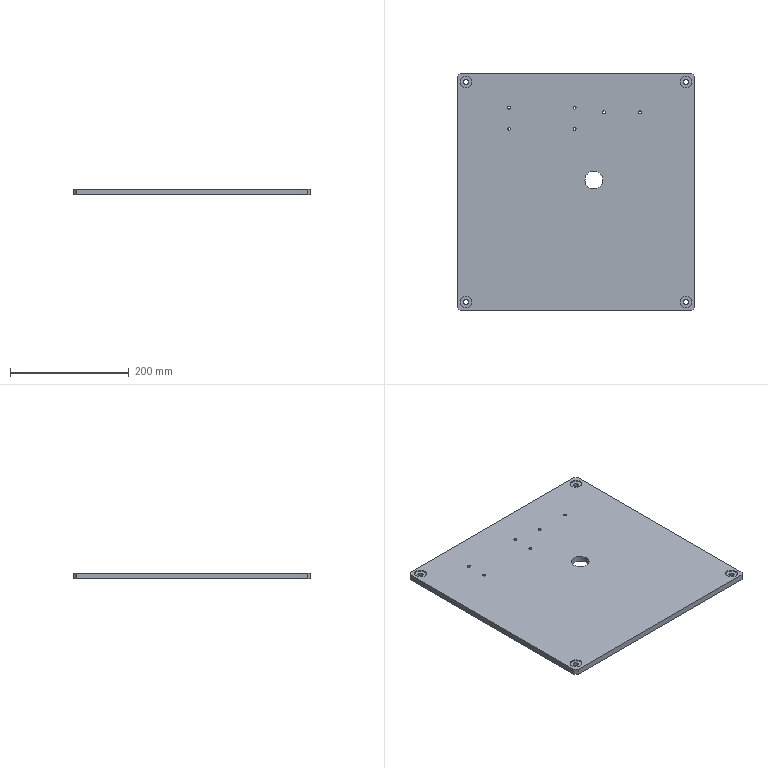Part | STEP file | 11-FG-SJ01811 | 1 solid | 44 faces | box 400 x 400 x 10 mm | volume 1586924 mm3 | cylinder 30 | plane 14 | commonest cylinder face diameters 5 x12 8.5 x8 20 x8 30 x2
STEP:
#1=CARTESIAN_POINT('',(-113.892,20.,0.));
#2=VERTEX_POINT('',#1);
#3=CARTESIAN_POINT('',(-83.892,20.,0.));
#4=VERTEX_POINT('',#3);
#5=CARTESIAN_POINT('',(-98.892,20.,0.));
#6=DIRECTION('',(0.,0.,1.));
#7=DIRECTION('',(1.,0.,0.));
#8=AXIS2_PLACEMENT_3D('',#5,#6,#7);
#9=CIRCLE('',#8,15.);
#10=EDGE_CURVE('',#2,#4,#9,.T.);
#11=ORIENTED_EDGE('',*,*,#10,.F.);
#12=CARTESIAN_POINT('',(-113.892,20.,10.));
#13=VERTEX_POINT('',#12);
#14=CARTESIAN_POINT('',(-113.892,20.,0.));
#15=DIRECTION('',(0.,0.,1.));
#16=VECTOR('',#15,1000.);
#17=LINE('',#14,#16);
#18=EDGE_CURVE('',#2,#13,#17,.T.);
#19=ORIENTED_EDGE('',*,*,#18,.T.);
#20=CARTESIAN_POINT('',(-83.892,20.,10.));
#21=VERTEX_POINT('',#20);
#22=CARTESIAN_POINT('',(-98.892,20.,10.));
#23=DIRECTION('',(0.,0.,1.));
#24=DIRECTION('',(1.,0.,0.));
#25=AXIS2_PLACEMENT_3D('',#22,#23,#24);
#26=CIRCLE('',#25,15.);
#27=EDGE_CURVE('',#13,#21,#26,.T.);
#28=ORIENTED_EDGE('',*,*,#27,.T.);
#29=CARTESIAN_POINT('',(-83.892,20.,0.));
#30=DIRECTION('',(0.,0.,1.));
#31=VECTOR('',#30,1000.);
#32=LINE('',#29,#31);
#33=EDGE_CURVE('',#4,#21,#32,.T.);
#34=ORIENTED_EDGE('',*,*,#33,.F.);
#35=EDGE_LOOP('',(#11,#19,#28,#34));
#36=FACE_OUTER_BOUND('',#35,.T.);
#37=CARTESIAN_POINT('',(-98.892,20.,0.));
#38=DIRECTION('',(0.,0.,1.));
#39=DIRECTION('',(1.,0.,0.));
#40=AXIS2_PLACEMENT_3D('',#37,#38,#39);
#41=CYLINDRICAL_SURFACE('',#40,15.);
#42=ADVANCED_FACE('',(#36),#41,.F.);
#43=CARTESIAN_POINT('',(-23.892,134.,0.));
#44=VERTEX_POINT('',#43);
#45=CARTESIAN_POINT('',(-18.892,134.,0.));
#46=VERTEX_POINT('',#45);
#47=CARTESIAN_POINT('',(-21.392,134.,0.));
#48=DIRECTION('',(0.,0.,1.));
#49=DIRECTION('',(1.,0.,0.));
#50=AXIS2_PLACEMENT_3D('',#47,#48,#49);
#51=CIRCLE('',#50,2.5);
#52=EDGE_CURVE('',#44,#46,#51,.T.);
#53=ORIENTED_EDGE('',*,*,#52,.F.);
#54=CARTESIAN_POINT('',(-23.892,134.,10.));
#55=VERTEX_POINT('',#54);
#56=CARTESIAN_POINT('',(-23.892,134.,10.));
#57=DIRECTION('',(0.,0.,1.));
#58=VECTOR('',#57,1000.);
#59=LINE('',#56,#58);
#60=EDGE_CURVE('',#44,#55,#59,.T.);
#61=ORIENTED_EDGE('',*,*,#60,.T.);
#62=CARTESIAN_POINT('',(-18.892,134.,10.));
#63=VERTEX_POINT('',#62);
#64=CARTESIAN_POINT('',(-21.392,134.,10.));
#65=DIRECTION('',(0.,0.,1.));
#66=DIRECTION('',(1.,0.,0.));
#67=AXIS2_PLACEMENT_3D('',#64,#65,#66);
#68=CIRCLE('',#67,2.5);
#69=EDGE_CURVE('',#55,#63,#68,.T.);
#70=ORIENTED_EDGE('',*,*,#69,.T.);
#71=CARTESIAN_POINT('',(-18.892,134.,10.));
#72=DIRECTION('',(0.,0.,1.));
#73=VECTOR('',#72,1000.);
#74=LINE('',#71,#73);
#75=EDGE_CURVE('',#46,#63,#74,.T.);
#76=ORIENTED_EDGE('',*,*,#75,.F.);
#77=EDGE_LOOP('',(#53,#61,#70,#76));
#78=FACE_OUTER_BOUND('',#77,.T.);
#79=CARTESIAN_POINT('',(-21.392,134.,10.));
#80=DIRECTION('',(0.,0.,1.));
#81=DIRECTION('',(1.,0.,0.));
#82=AXIS2_PLACEMENT_3D('',#79,#80,#81);
#83=CYLINDRICAL_SURFACE('',#82,2.5);
#84=ADVANCED_FACE('',(#78),#83,.F.);
#85=CARTESIAN_POINT('',(-83.892,134.,0.));
#86=VERTEX_POINT('',#85);
#87=CARTESIAN_POINT('',(-78.892,134.,0.));
#88=VERTEX_POINT('',#87);
#89=CARTESIAN_POINT('',(-81.392,134.,0.));
#90=DIRECTION('',(0.,0.,1.));
#91=DIRECTION('',(1.,0.,0.));
#92=AXIS2_PLACEMENT_3D('',#89,#90,#91);
#93=CIRCLE('',#92,2.5);
#94=EDGE_CURVE('',#86,#88,#93,.T.);
#95=ORIENTED_EDGE('',*,*,#94,.F.);
#96=CARTESIAN_POINT('',(-83.892,134.,10.));
#97=VERTEX_POINT('',#96);
#98=CARTESIAN_POINT('',(-83.892,134.,10.));
#99=DIRECTION('',(0.,0.,1.));
#100=VECTOR('',#99,1000.);
#101=LINE('',#98,#100);
#102=EDGE_CURVE('',#86,#97,#101,.T.);
#103=ORIENTED_EDGE('',*,*,#102,.T.);
#104=CARTESIAN_POINT('',(-78.892,134.,10.));
#105=VERTEX_POINT('',#104);
#106=CARTESIAN_POINT('',(-81.392,134.,10.));
#107=DIRECTION('',(0.,0.,1.));
#108=DIRECTION('',(1.,0.,0.));
#109=AXIS2_PLACEMENT_3D('',#106,#107,#108);
#110=CIRCLE('',#109,2.5);
#111=EDGE_CURVE('',#97,#105,#110,.T.);
#112=ORIENTED_EDGE('',*,*,#111,.T.);
#113=CARTESIAN_POINT('',(-78.892,134.,10.));
#114=DIRECTION('',(0.,0.,1.));
#115=VECTOR('',#114,1000.);
#116=LINE('',#113,#115);
#117=EDGE_CURVE('',#88,#105,#116,.T.);
#118=ORIENTED_EDGE('',*,*,#117,.F.);
#119=EDGE_LOOP('',(#95,#103,#112,#118));
#120=FACE_OUTER_BOUND('',#119,.T.);
#121=CARTESIAN_POINT('',(-81.392,134.,10.));
#122=DIRECTION('',(0.,0.,1.));
#123=DIRECTION('',(1.,0.,0.));
#124=AXIS2_PLACEMENT_3D('',#121,#122,#123);
#125=CYLINDRICAL_SURFACE('',#124,2.5);
#126=ADVANCED_FACE('',(#120),#125,.F.);
#127=CARTESIAN_POINT('',(-133.892,142.,0.));
#128=VERTEX_POINT('',#127);
#129=CARTESIAN_POINT('',(-128.892,142.,0.));
#130=VERTEX_POINT('',#129);
#131=CARTESIAN_POINT('',(-131.392,142.,0.));
#132=DIRECTION('',(0.,0.,1.));
#133=DIRECTION('',(1.,0.,0.));
#134=AXIS2_PLACEMENT_3D('',#131,#132,#133);
#135=CIRCLE('',#134,2.5);
#136=EDGE_CURVE('',#128,#130,#135,.T.);
#137=ORIENTED_EDGE('',*,*,#136,.F.);
#138=CARTESIAN_POINT('',(-133.892,142.,10.));
#139=VERTEX_POINT('',#138);
#140=CARTESIAN_POINT('',(-133.892,142.,10.));
#141=DIRECTION('',(0.,0.,1.));
#142=VECTOR('',#141,1000.);
#143=LINE('',#140,#142);
#144=EDGE_CURVE('',#128,#139,#143,.T.);
#145=ORIENTED_EDGE('',*,*,#144,.T.);
#146=CARTESIAN_POINT('',(-128.892,142.,10.));
#147=VERTEX_POINT('',#146);
#148=CARTESIAN_POINT('',(-131.392,142.,10.));
#149=DIRECTION('',(0.,0.,1.));
#150=DIRECTION('',(1.,0.,0.));
#151=AXIS2_PLACEMENT_3D('',#148,#149,#150);
#152=CIRCLE('',#151,2.5);
#153=EDGE_CURVE('',#139,#147,#152,.T.);
#154=ORIENTED_EDGE('',*,*,#153,.T.);
#155=CARTESIAN_POINT('',(-128.892,142.,10.));
#156=DIRECTION('',(0.,0.,1.));
#157=VECTOR('',#156,1000.);
#158=LINE('',#155,#157);
#159=EDGE_CURVE('',#130,#147,#158,.T.);
#160=ORIENTED_EDGE('',*,*,#159,.F.);
#161=EDGE_LOOP('',(#137,#145,#154,#160));
#162=FACE_OUTER_BOUND('',#161,.T.);
#163=CARTESIAN_POINT('',(-131.392,142.,10.));
#164=DIRECTION('',(0.,0.,1.));
#165=DIRECTION('',(1.,0.,0.));
#166=AXIS2_PLACEMENT_3D('',#163,#164,#165);
#167=CYLINDRICAL_SURFACE('',#166,2.5);
#168=ADVANCED_FACE('',(#162),#167,.F.);
#169=CARTESIAN_POINT('',(-133.892,106.,0.));
#170=VERTEX_POINT('',#169);
#171=CARTESIAN_POINT('',(-128.892,106.,0.));
#172=VERTEX_POINT('',#171);
#173=CARTESIAN_POINT('',(-131.392,106.,0.));
#174=DIRECTION('',(0.,0.,1.));
#175=DIRECTION('',(1.,0.,0.));
#176=AXIS2_PLACEMENT_3D('',#173,#174,#175);
#177=CIRCLE('',#176,2.5);
#178=EDGE_CURVE('',#170,#172,#177,.T.);
#179=ORIENTED_EDGE('',*,*,#178,.F.);
#180=CARTESIAN_POINT('',(-133.892,106.,10.));
#181=VERTEX_POINT('',#180);
#182=CARTESIAN_POINT('',(-133.892,106.,10.));
#183=DIRECTION('',(0.,0.,1.));
#184=VECTOR('',#183,1000.);
#185=LINE('',#182,#184);
#186=EDGE_CURVE('',#170,#181,#185,.T.);
#187=ORIENTED_EDGE('',*,*,#186,.T.);
#188=CARTESIAN_POINT('',(-128.892,106.,10.));
#189=VERTEX_POINT('',#188);
#190=CARTESIAN_POINT('',(-131.392,106.,10.));
#191=DIRECTION('',(0.,0.,1.));
#192=DIRECTION('',(1.,0.,0.));
#193=AXIS2_PLACEMENT_3D('',#190,#191,#192);
#194=CIRCLE('',#193,2.5);
#195=EDGE_CURVE('',#181,#189,#194,.T.);
#196=ORIENTED_EDGE('',*,*,#195,.T.);
#197=CARTESIAN_POINT('',(-128.892,106.,10.));
#198=DIRECTION('',(0.,0.,1.));
#199=VECTOR('',#198,1000.);
#200=LINE('',#197,#199);
#201=EDGE_CURVE('',#172,#189,#200,.T.);
#202=ORIENTED_EDGE('',*,*,#201,.F.);
#203=EDGE_LOOP('',(#179,#187,#196,#202));
#204=FACE_OUTER_BOUND('',#203,.T.);
#205=CARTESIAN_POINT('',(-131.392,106.,10.));
#206=DIRECTION('',(0.,0.,1.));
#207=DIRECTION('',(1.,0.,0.));
#208=AXIS2_PLACEMENT_3D('',#205,#206,#207);
#209=CYLINDRICAL_SURFACE('',#208,2.5);
#210=ADVANCED_FACE('',(#204),#209,.F.);
#211=CARTESIAN_POINT('',(-243.892,106.,0.));
#212=VERTEX_POINT('',#211);
#213=CARTESIAN_POINT('',(-238.892,106.,0.));
#214=VERTEX_POINT('',#213);
#215=CARTESIAN_POINT('',(-241.392,106.,0.));
#216=DIRECTION('',(0.,0.,1.));
#217=DIRECTION('',(1.,0.,0.));
#218=AXIS2_PLACEMENT_3D('',#215,#216,#217);
#219=CIRCLE('',#218,2.5);
#220=EDGE_CURVE('',#212,#214,#219,.T.);
#221=ORIENTED_EDGE('',*,*,#220,.F.);
#222=CARTESIAN_POINT('',(-243.892,106.,10.));
#223=VERTEX_POINT('',#222);
#224=CARTESIAN_POINT('',(-243.892,106.,10.));
#225=DIRECTION('',(0.,0.,1.));
#226=VECTOR('',#225,1000.);
#227=LINE('',#224,#226);
#228=EDGE_CURVE('',#212,#223,#227,.T.);
#229=ORIENTED_EDGE('',*,*,#228,.T.);
#230=CARTESIAN_POINT('',(-238.892,106.,10.));
#231=VERTEX_POINT('',#230);
#232=CARTESIAN_POINT('',(-241.392,106.,10.));
#233=DIRECTION('',(0.,0.,1.));
#234=DIRECTION('',(1.,0.,0.));
#235=AXIS2_PLACEMENT_3D('',#232,#233,#234);
#236=CIRCLE('',#235,2.5);
#237=EDGE_CURVE('',#223,#231,#236,.T.);
#238=ORIENTED_EDGE('',*,*,#237,.T.);
#239=CARTESIAN_POINT('',(-238.892,106.,10.));
#240=DIRECTION('',(0.,0.,1.));
#241=VECTOR('',#240,1000.);
#242=LINE('',#239,#241);
#243=EDGE_CURVE('',#214,#231,#242,.T.);
#244=ORIENTED_EDGE('',*,*,#243,.F.);
#245=EDGE_LOOP('',(#221,#229,#238,#244));
#246=FACE_OUTER_BOUND('',#245,.T.);
#247=CARTESIAN_POINT('',(-241.392,106.,10.));
#248=DIRECTION('',(0.,0.,1.));
#249=DIRECTION('',(1.,0.,0.));
#250=AXIS2_PLACEMENT_3D('',#247,#248,#249);
#251=CYLINDRICAL_SURFACE('',#250,2.5);
#252=ADVANCED_FACE('',(#246),#251,.F.);
#253=CARTESIAN_POINT('',(-243.892,142.,0.));
#254=VERTEX_POINT('',#253);
#255=CARTESIAN_POINT('',(-238.892,142.,0.));
#256=VERTEX_POINT('',#255);
#257=CARTESIAN_POINT('',(-241.392,142.,0.));
#258=DIRECTION('',(0.,0.,1.));
#259=DIRECTION('',(1.,0.,0.));
#260=AXIS2_PLACEMENT_3D('',#257,#258,#259);
#261=CIRCLE('',#260,2.5);
#262=EDGE_CURVE('',#254,#256,#261,.T.);
#263=ORIENTED_EDGE('',*,*,#262,.F.);
#264=CARTESIAN_POINT('',(-243.892,142.,10.));
#265=VERTEX_POINT('',#264);
#266=CARTESIAN_POINT('',(-243.892,142.,10.));
#267=DIRECTION('',(0.,0.,1.));
#268=VECTOR('',#267,1000.);
#269=LINE('',#266,#268);
#270=EDGE_CURVE('',#254,#265,#269,.T.);
#271=ORIENTED_EDGE('',*,*,#270,.T.);
#272=CARTESIAN_POINT('',(-238.892,142.,10.));
#273=VERTEX_POINT('',#272);
#274=CARTESIAN_POINT('',(-241.392,142.,10.));
#275=DIRECTION('',(0.,0.,1.));
#276=DIRECTION('',(1.,0.,0.));
#277=AXIS2_PLACEMENT_3D('',#274,#275,#276);
#278=CIRCLE('',#277,2.5);
#279=EDGE_CURVE('',#265,#273,#278,.T.);
#280=ORIENTED_EDGE('',*,*,#279,.T.);
#281=CARTESIAN_POINT('',(-238.892,142.,10.));
#282=DIRECTION('',(0.,0.,1.));
#283=VECTOR('',#282,1000.);
#284=LINE('',#281,#283);
#285=EDGE_CURVE('',#256,#273,#284,.T.);
#286=ORIENTED_EDGE('',*,*,#285,.F.);
#287=EDGE_LOOP('',(#263,#271,#280,#286));
#288=FACE_OUTER_BOUND('',#287,.T.);
#289=CARTESIAN_POINT('',(-241.392,142.,10.));
#290=DIRECTION('',(0.,0.,1.));
#291=DIRECTION('',(1.,0.,0.));
#292=AXIS2_PLACEMENT_3D('',#289,#290,#291);
#293=CYLINDRICAL_SURFACE('',#292,2.5);
#294=ADVANCED_FACE('',(#288),#293,.F.);
#295=CARTESIAN_POINT('',(-318.142,-185.,0.));
#296=VERTEX_POINT('',#295);
#297=CARTESIAN_POINT('',(-309.642,-185.,0.));
#298=VERTEX_POINT('',#297);
#299=CARTESIAN_POINT('',(-313.892,-185.,0.));
#300=DIRECTION('',(0.,0.,1.));
#301=DIRECTION('',(1.,0.,0.));
#302=AXIS2_PLACEMENT_3D('',#299,#300,#301);
#303=CIRCLE('',#302,4.25);
#304=EDGE_CURVE('',#296,#298,#303,.T.);
#305=ORIENTED_EDGE('',*,*,#304,.F.);
#306=CARTESIAN_POINT('',(-318.142,-185.,8.));
#307=VERTEX_POINT('',#306);
#308=CARTESIAN_POINT('',(-318.142,-185.,0.));
#309=DIRECTION('',(0.,0.,1.));
#310=VECTOR('',#309,1000.);
#311=LINE('',#308,#310);
#312=EDGE_CURVE('',#296,#307,#311,.T.);
#313=ORIENTED_EDGE('',*,*,#312,.T.);
#314=CARTESIAN_POINT('',(-309.642,-185.,8.));
#315=VERTEX_POINT('',#314);
#316=CARTESIAN_POINT('',(-313.892,-185.,8.));
#317=DIRECTION('',(0.,0.,-1.));
#318=DIRECTION('',(-1.,0.,0.));
#319=AXIS2_PLACEMENT_3D('',#316,#317,#318);
#320=CIRCLE('',#319,4.25);
#321=EDGE_CURVE('',#315,#307,#320,.T.);
#322=ORIENTED_EDGE('',*,*,#321,.F.);
#323=CARTESIAN_POINT('',(-309.642,-185.,0.));
#324=DIRECTION('',(0.,0.,1.));
#325=VECTOR('',#324,1000.);
#326=LINE('',#323,#325);
#327=EDGE_CURVE('',#298,#315,#326,.T.);
#328=ORIENTED_EDGE('',*,*,#327,.F.);
#329=EDGE_LOOP('',(#305,#313,#322,#328));
#330=FACE_OUTER_BOUND('',#329,.T.);
#331=CARTESIAN_POINT('',(-313.892,-185.,0.));
#332=DIRECTION('',(0.,0.,1.));
#333=DIRECTION('',(1.,0.,0.));
#334=AXIS2_PLACEMENT_3D('',#331,#332,#333);
#335=CYLINDRICAL_SURFACE('',#334,4.25);
#336=ADVANCED_FACE('',(#330),#335,.F.);
#337=CARTESIAN_POINT('',(51.858,-185.,0.));
#338=VERTEX_POINT('',#337);
#339=CARTESIAN_POINT('',(60.358,-185.,0.));
#340=VERTEX_POINT('',#339);
#341=CARTESIAN_POINT('',(56.108,-185.,0.));
#342=DIRECTION('',(0.,0.,1.));
#343=DIRECTION('',(1.,0.,0.));
#344=AXIS2_PLACEMENT_3D('',#341,#342,#343);
#345=CIRCLE('',#344,4.25);
#346=EDGE_CURVE('',#338,#340,#345,.T.);
#347=ORIENTED_EDGE('',*,*,#346,.F.);
#348=CARTESIAN_POINT('',(51.858,-185.,8.));
#349=VERTEX_POINT('',#348);
#350=CARTESIAN_POINT('',(51.858,-185.,0.));
#351=DIRECTION('',(0.,0.,1.));
#352=VECTOR('',#351,1000.);
#353=LINE('',#350,#352);
#354=EDGE_CURVE('',#338,#349,#353,.T.);
#355=ORIENTED_EDGE('',*,*,#354,.T.);
#356=CARTESIAN_POINT('',(60.358,-185.,8.));
#357=VERTEX_POINT('',#356);
#358=CARTESIAN_POINT('',(56.108,-185.,8.));
#359=DIRECTION('',(0.,0.,1.));
#360=DIRECTION('',(1.,0.,0.));
#361=AXIS2_PLACEMENT_3D('',#358,#359,#360);
#362=CIRCLE('',#361,4.25);
#363=EDGE_CURVE('',#349,#357,#362,.T.);
#364=ORIENTED_EDGE('',*,*,#363,.T.);
#365=CARTESIAN_POINT('',(60.358,-185.,0.));
#366=DIRECTION('',(0.,0.,1.));
#367=VECTOR('',#366,1000.);
#368=LINE('',#365,#367);
#369=EDGE_CURVE('',#340,#357,#368,.T.);
#370=ORIENTED_EDGE('',*,*,#369,.F.);
#371=EDGE_LOOP('',(#347,#355,#364,#370));
#372=FACE_OUTER_BOUND('',#371,.T.);
#373=CARTESIAN_POINT('',(56.108,-185.,0.));
#374=DIRECTION('',(0.,0.,1.));
#375=DIRECTION('',(1.,0.,0.));
#376=AXIS2_PLACEMENT_3D('',#373,#374,#375);
#377=CYLINDRICAL_SURFACE('',#376,4.25);
#378=ADVANCED_FACE('',(#372),#377,.F.);
#379=CARTESIAN_POINT('',(51.858,185.,0.));
#380=VERTEX_POINT('',#379);
#381=CARTESIAN_POINT('',(60.358,185.,0.));
#382=VERTEX_POINT('',#381);
#383=CARTESIAN_POINT('',(56.108,185.,0.));
#384=DIRECTION('',(0.,0.,1.));
#385=DIRECTION('',(1.,0.,0.));
#386=AXIS2_PLACEMENT_3D('',#383,#384,#385);
#387=CIRCLE('',#386,4.25);
#388=EDGE_CURVE('',#380,#382,#387,.T.);
#389=ORIENTED_EDGE('',*,*,#388,.F.);
#390=CARTESIAN_POINT('',(51.858,185.,8.));
#391=VERTEX_POINT('',#390);
#392=CARTESIAN_POINT('',(51.858,185.,0.));
#393=DIRECTION('',(0.,0.,1.));
#394=VECTOR('',#393,1000.);
#395=LINE('',#392,#394);
#396=EDGE_CURVE('',#380,#391,#395,.T.);
#397=ORIENTED_EDGE('',*,*,#396,.T.);
#398=CARTESIAN_POINT('',(60.358,185.,8.));
#399=VERTEX_POINT('',#398);
#400=CARTESIAN_POINT('',(56.108,185.,8.));
#401=DIRECTION('',(0.,0.,-1.));
#402=DIRECTION('',(-1.,0.,0.));
#403=AXIS2_PLACEMENT_3D('',#400,#401,#402);
#404=CIRCLE('',#403,4.25);
#405=EDGE_CURVE('',#399,#391,#404,.T.);
#406=ORIENTED_EDGE('',*,*,#405,.F.);
#407=CARTESIAN_POINT('',(60.358,185.,0.));
#408=DIRECTION('',(0.,0.,1.));
#409=VECTOR('',#408,1000.);
#410=LINE('',#407,#409);
#411=EDGE_CURVE('',#382,#399,#410,.T.);
#412=ORIENTED_EDGE('',*,*,#411,.F.);
#413=EDGE_LOOP('',(#389,#397,#406,#412));
#414=FACE_OUTER_BOUND('',#413,.T.);
#415=CARTESIAN_POINT('',(56.108,185.,0.));
#416=DIRECTION('',(0.,0.,1.));
#417=DIRECTION('',(1.,0.,0.));
#418=AXIS2_PLACEMENT_3D('',#415,#416,#417);
#419=CYLINDRICAL_SURFACE('',#418,4.25);
#420=ADVANCED_FACE('',(#414),#419,.F.);
#421=CARTESIAN_POINT('',(-318.142,185.,0.));
#422=VERTEX_POINT('',#421);
#423=CARTESIAN_POINT('',(-309.642,185.,0.));
#424=VERTEX_POINT('',#423);
#425=CARTESIAN_POINT('',(-313.892,185.,0.));
#426=DIRECTION('',(0.,0.,1.));
#427=DIRECTION('',(1.,0.,0.));
#428=AXIS2_PLACEMENT_3D('',#425,#426,#427);
#429=CIRCLE('',#428,4.25);
#430=EDGE_CURVE('',#422,#424,#429,.T.);
#431=ORIENTED_EDGE('',*,*,#430,.F.);
#432=CARTESIAN_POINT('',(-318.142,185.,8.));
#433=VERTEX_POINT('',#432);
#434=CARTESIAN_POINT('',(-318.142,185.,0.));
#435=DIRECTION('',(0.,0.,1.));
#436=VECTOR('',#435,1000.);
#437=LINE('',#434,#436);
#438=EDGE_CURVE('',#422,#433,#437,.T.);
#439=ORIENTED_EDGE('',*,*,#438,.T.);
#440=CARTESIAN_POINT('',(-309.642,185.,8.));
#441=VERTEX_POINT('',#440);
#442=CARTESIAN_POINT('',(-313.892,185.,8.));
#443=DIRECTION('',(0.,0.,1.));
#444=DIRECTION('',(1.,0.,0.));
#445=AXIS2_PLACEMENT_3D('',#442,#443,#444);
#446=CIRCLE('',#445,4.25);
#447=EDGE_CURVE('',#433,#441,#446,.T.);
#448=ORIENTED_EDGE('',*,*,#447,.T.);
#449=CARTESIAN_POINT('',(-309.642,185.,0.));
#450=DIRECTION('',(0.,0.,1.));
#451=VECTOR('',#450,1000.);
#452=LINE('',#449,#451);
#453=EDGE_CURVE('',#424,#441,#452,.T.);
#454=ORIENTED_EDGE('',*,*,#453,.F.);
#455=EDGE_LOOP('',(#431,#439,#448,#454));
#456=FACE_OUTER_BOUND('',#455,.T.);
#457=CARTESIAN_POINT('',(-313.892,185.,0.));
#458=DIRECTION('',(0.,0.,1.));
#459=DIRECTION('',(1.,0.,0.));
#460=AXIS2_PLACEMENT_3D('',#457,#458,#459);
#461=CYLINDRICAL_SURFACE('',#460,4.25);
#462=ADVANCED_FACE('',(#456),#461,.F.);
#463=CARTESIAN_POINT('',(46.108,185.,8.));
#464=VERTEX_POINT('',#463);
#465=CARTESIAN_POINT('',(66.108,185.,8.));
#466=VERTEX_POINT('',#465);
#467=CARTESIAN_POINT('',(56.108,185.,8.));
#468=DIRECTION('',(0.,0.,1.));
#469=DIRECTION('',(-1.,0.,0.));
#470=AXIS2_PLACEMENT_3D('',#467,#468,#469);
#471=CIRCLE('',#470,10.);
#472=EDGE_CURVE('',#464,#466,#471,.T.);
#473=ORIENTED_EDGE('',*,*,#472,.F.);
#474=CARTESIAN_POINT('',(46.108,185.,10.));
#475=VERTEX_POINT('',#474);
#476=CARTESIAN_POINT('',(46.108,185.,8.));
#477=DIRECTION('',(0.,0.,1.));
#478=VECTOR('',#477,1000.);
#479=LINE('',#476,#478);
#480=EDGE_CURVE('',#464,#475,#479,.T.);
#481=ORIENTED_EDGE('',*,*,#480,.T.);
#482=CARTESIAN_POINT('',(66.108,185.,10.));
#483=VERTEX_POINT('',#482);
#484=CARTESIAN_POINT('',(56.108,185.,10.));
#485=DIRECTION('',(0.,0.,1.));
#486=DIRECTION('',(-1.,0.,0.));
#487=AXIS2_PLACEMENT_3D('',#484,#485,#486);
#488=CIRCLE('',#487,10.);
#489=EDGE_CURVE('',#475,#483,#488,.T.);
#490=ORIENTED_EDGE('',*,*,#489,.T.);
#491=CARTESIAN_POINT('',(66.108,185.,8.));
#492=DIRECTION('',(0.,0.,1.));
#493=VECTOR('',#492,1000.);
#494=LINE('',#491,#493);
#495=EDGE_CURVE('',#466,#483,#494,.T.);
#496=ORIENTED_EDGE('',*,*,#495,.F.);
#497=EDGE_LOOP('',(#473,#481,#490,#496));
#498=FACE_OUTER_BOUND('',#497,.T.);
#499=CARTESIAN_POINT('',(56.108,185.,8.));
#500=DIRECTION('',(0.,0.,1.));
#501=DIRECTION('',(1.,0.,0.));
#502=AXIS2_PLACEMENT_3D('',#499,#500,#501);
#503=CYLINDRICAL_SURFACE('',#502,10.);
#504=ADVANCED_FACE('',(#498),#503,.F.);
#505=CARTESIAN_POINT('',(46.108,-185.,8.));
#506=VERTEX_POINT('',#505);
#507=CARTESIAN_POINT('',(66.108,-185.,8.));
#508=VERTEX_POINT('',#507);
#509=CARTESIAN_POINT('',(56.108,-185.,8.));
#510=DIRECTION('',(0.,0.,1.));
#511=DIRECTION('',(1.,0.,0.));
#512=AXIS2_PLACEMENT_3D('',#509,#510,#511);
#513=CIRCLE('',#512,10.);
#514=EDGE_CURVE('',#506,#508,#513,.T.);
#515=ORIENTED_EDGE('',*,*,#514,.F.);
#516=CARTESIAN_POINT('',(46.108,-185.,10.));
#517=VERTEX_POINT('',#516);
#518=CARTESIAN_POINT('',(46.108,-185.,8.));
#519=DIRECTION('',(0.,0.,1.));
#520=VECTOR('',#519,1000.);
#521=LINE('',#518,#520);
#522=EDGE_CURVE('',#506,#517,#521,.T.);
#523=ORIENTED_EDGE('',*,*,#522,.T.);
#524=CARTESIAN_POINT('',(66.108,-185.,10.));
#525=VERTEX_POINT('',#524);
#526=CARTESIAN_POINT('',(56.108,-185.,10.));
#527=DIRECTION('',(0.,0.,1.));
#528=DIRECTION('',(1.,0.,0.));
#529=AXIS2_PLACEMENT_3D('',#526,#527,#528);
#530=CIRCLE('',#529,10.);
#531=EDGE_CURVE('',#517,#525,#530,.T.);
#532=ORIENTED_EDGE('',*,*,#531,.T.);
#533=CARTESIAN_POINT('',(66.108,-185.,8.));
#534=DIRECTION('',(0.,0.,1.));
#535=VECTOR('',#534,1000.);
#536=LINE('',#533,#535);
#537=EDGE_CURVE('',#508,#525,#536,.T.);
#538=ORIENTED_EDGE('',*,*,#537,.F.);
#539=EDGE_LOOP('',(#515,#523,#532,#538));
#540=FACE_OUTER_BOUND('',#539,.T.);
#541=CARTESIAN_POINT('',(56.108,-185.,8.));
#542=DIRECTION('',(0.,0.,1.));
#543=DIRECTION('',(1.,0.,0.));
#544=AXIS2_PLACEMENT_3D('',#541,#542,#543);
#545=CYLINDRICAL_SURFACE('',#544,10.);
#546=ADVANCED_FACE('',(#540),#545,.F.);
#547=CARTESIAN_POINT('',(-323.892,-185.,8.));
#548=VERTEX_POINT('',#547);
#549=CARTESIAN_POINT('',(-303.892,-185.,8.));
#550=VERTEX_POINT('',#549);
#551=CARTESIAN_POINT('',(-313.892,-185.,8.));
#552=DIRECTION('',(0.,0.,1.));
#553=DIRECTION('',(-1.,0.,0.));
#554=AXIS2_PLACEMENT_3D('',#551,#552,#553);
#555=CIRCLE('',#554,10.);
#556=EDGE_CURVE('',#548,#550,#555,.T.);
#557=ORIENTED_EDGE('',*,*,#556,.F.);
#558=CARTESIAN_POINT('',(-323.892,-185.,10.));
#559=VERTEX_POINT('',#558);
#560=CARTESIAN_POINT('',(-323.892,-185.,8.));
#561=DIRECTION('',(0.,0.,1.));
#562=VECTOR('',#561,1000.);
#563=LINE('',#560,#562);
#564=EDGE_CURVE('',#548,#559,#563,.T.);
#565=ORIENTED_EDGE('',*,*,#564,.T.);
#566=CARTESIAN_POINT('',(-303.892,-185.,10.));
#567=VERTEX_POINT('',#566);
#568=CARTESIAN_POINT('',(-313.892,-185.,10.));
#569=DIRECTION('',(0.,0.,1.));
#570=DIRECTION('',(-1.,0.,0.));
#571=AXIS2_PLACEMENT_3D('',#568,#569,#570);
#572=CIRCLE('',#571,10.);
#573=EDGE_CURVE('',#559,#567,#572,.T.);
#574=ORIENTED_EDGE('',*,*,#573,.T.);
#575=CARTESIAN_POINT('',(-303.892,-185.,8.));
#576=DIRECTION('',(0.,0.,1.));
#577=VECTOR('',#576,1000.);
#578=LINE('',#575,#577);
#579=EDGE_CURVE('',#550,#567,#578,.T.);
#580=ORIENTED_EDGE('',*,*,#579,.F.);
#581=EDGE_LOOP('',(#557,#565,#574,#580));
#582=FACE_OUTER_BOUND('',#581,.T.);
#583=CARTESIAN_POINT('',(-313.892,-185.,8.));
#584=DIRECTION('',(0.,0.,1.));
#585=DIRECTION('',(1.,0.,0.));
#586=AXIS2_PLACEMENT_3D('',#583,#584,#585);
#587=CYLINDRICAL_SURFACE('',#586,10.);
#588=ADVANCED_FACE('',(#582),#587,.F.);
#589=CARTESIAN_POINT('',(-323.892,185.,8.));
#590=VERTEX_POINT('',#589);
#591=CARTESIAN_POINT('',(-303.892,185.,8.));
#592=VERTEX_POINT('',#591);
#593=CARTESIAN_POINT('',(-313.892,185.,8.));
#594=DIRECTION('',(0.,0.,1.));
#595=DIRECTION('',(1.,0.,0.));
#596=AXIS2_PLACEMENT_3D('',#593,#594,#595);
#597=CIRCLE('',#596,10.);
#598=EDGE_CURVE('',#590,#592,#597,.T.);
#599=ORIENTED_EDGE('',*,*,#598,.F.);
#600=CARTESIAN_POINT('',(-323.892,185.,10.));
#601=VERTEX_POINT('',#600);
#602=CARTESIAN_POINT('',(-323.892,185.,8.));
#603=DIRECTION('',(0.,0.,1.));
#604=VECTOR('',#603,1000.);
#605=LINE('',#602,#604);
#606=EDGE_CURVE('',#590,#601,#605,.T.);
#607=ORIENTED_EDGE('',*,*,#606,.T.);
#608=CARTESIAN_POINT('',(-303.892,185.,10.));
#609=VERTEX_POINT('',#608);
#610=CARTESIAN_POINT('',(-313.892,185.,10.));
#611=DIRECTION('',(0.,0.,1.));
#612=DIRECTION('',(1.,0.,0.));
#613=AXIS2_PLACEMENT_3D('',#610,#611,#612);
#614=CIRCLE('',#613,10.);
#615=EDGE_CURVE('',#601,#609,#614,.T.);
#616=ORIENTED_EDGE('',*,*,#615,.T.);
#617=CARTESIAN_POINT('',(-303.892,185.,8.));
#618=DIRECTION('',(0.,0.,1.));
#619=VECTOR('',#618,1000.);
#620=LINE('',#617,#619);
#621=EDGE_CURVE('',#592,#609,#620,.T.);
#622=ORIENTED_EDGE('',*,*,#621,.F.);
#623=EDGE_LOOP('',(#599,#607,#616,#622));
#624=FACE_OUTER_BOUND('',#623,.T.);
#625=CARTESIAN_POINT('',(-313.892,185.,8.));
#626=DIRECTION('',(0.,0.,1.));
#627=DIRECTION('',(1.,0.,0.));
#628=AXIS2_PLACEMENT_3D('',#625,#626,#627);
#629=CYLINDRICAL_SURFACE('',#628,10.);
#630=ADVANCED_FACE('',(#624),#629,.F.);
#631=CARTESIAN_POINT('',(71.108,-195.,10.));
#632=VERTEX_POINT('',#631);
#633=CARTESIAN_POINT('',(71.108,195.,10.));
#634=VERTEX_POINT('',#633);
#635=CARTESIAN_POINT('',(71.108,-200.,10.));
#636=DIRECTION('',(0.,1.,0.));
#637=VECTOR('',#636,1000.);
#638=LINE('',#635,#637);
#639=EDGE_CURVE('',#632,#634,#638,.T.);
#640=ORIENTED_EDGE('',*,*,#639,.F.);
#641=CARTESIAN_POINT('',(71.108,-195.,0.));
#642=VERTEX_POINT('',#641);
#643=CARTESIAN_POINT('',(71.108,-195.,10.));
#644=DIRECTION('',(0.,0.,-1.));
#645=VECTOR('',#644,1000.);
#646=LINE('',#643,#645);
#647=EDGE_CURVE('',#632,#642,#646,.T.);
#648=ORIENTED_EDGE('',*,*,#647,.T.);
#649=CARTESIAN_POINT('',(71.108,195.,0.));
#650=VERTEX_POINT('',#649);
#651=CARTESIAN_POINT('',(71.108,-200.,0.));
#652=DIRECTION('',(0.,1.,0.));
#653=VECTOR('',#652,1000.);
#654=LINE('',#651,#653);
#655=EDGE_CURVE('',#642,#650,#654,.T.);
#656=ORIENTED_EDGE('',*,*,#655,.T.);
#657=CARTESIAN_POINT('',(71.108,195.,10.));
#658=DIRECTION('',(0.,0.,1.));
#659=VECTOR('',#658,1000.);
#660=LINE('',#657,#659);
#661=EDGE_CURVE('',#650,#634,#660,.T.);
#662=ORIENTED_EDGE('',*,*,#661,.T.);
#663=EDGE_LOOP('',(#640,#648,#656,#662));
#664=FACE_OUTER_BOUND('',#663,.T.);
#665=CARTESIAN_POINT('',(71.108,-200.,10.));
#666=DIRECTION('',(-1.,0.,0.));
#667=DIRECTION('',(0.,0.,1.));
#668=AXIS2_PLACEMENT_3D('',#665,#666,#667);
#669=PLANE('',#668);
#670=ADVANCED_FACE('',(#664),#669,.F.);
#671=CARTESIAN_POINT('',(66.108,200.,10.));
#672=VERTEX_POINT('',#671);
#673=CARTESIAN_POINT('',(-323.892,200.,10.));
#674=VERTEX_POINT('',#673);
#675=CARTESIAN_POINT('',(71.108,200.,10.));
#676=DIRECTION('',(-1.,0.,0.));
#677=VECTOR('',#676,1000.);
#678=LINE('',#675,#677);
#679=EDGE_CURVE('',#672,#674,#678,.T.);
#680=ORIENTED_EDGE('',*,*,#679,.F.);
#681=CARTESIAN_POINT('',(66.108,200.,0.));
#682=VERTEX_POINT('',#681);
#683=CARTESIAN_POINT('',(66.108,200.,10.));
#684=DIRECTION('',(0.,0.,-1.));
#685=VECTOR('',#684,1000.);
#686=LINE('',#683,#685);
#687=EDGE_CURVE('',#672,#682,#686,.T.);
#688=ORIENTED_EDGE('',*,*,#687,.T.);
#689=CARTESIAN_POINT('',(-323.892,200.,0.));
#690=VERTEX_POINT('',#689);
#691=CARTESIAN_POINT('',(71.108,200.,0.));
#692=DIRECTION('',(-1.,0.,0.));
#693=VECTOR('',#692,1000.);
#694=LINE('',#691,#693);
#695=EDGE_CURVE('',#682,#690,#694,.T.);
#696=ORIENTED_EDGE('',*,*,#695,.T.);
#697=CARTESIAN_POINT('',(-323.892,200.,10.));
#698=DIRECTION('',(0.,0.,1.));
#699=VECTOR('',#698,1000.);
#700=LINE('',#697,#699);
#701=EDGE_CURVE('',#690,#674,#700,.T.);
#702=ORIENTED_EDGE('',*,*,#701,.T.);
#703=EDGE_LOOP('',(#680,#688,#696,#702));
#704=FACE_OUTER_BOUND('',#703,.T.);
#705=CARTESIAN_POINT('',(71.108,200.,10.));
#706=DIRECTION('',(0.,-1.,0.));
#707=DIRECTION('',(1.,0.,0.));
#708=AXIS2_PLACEMENT_3D('',#705,#706,#707);
#709=PLANE('',#708);
#710=ADVANCED_FACE('',(#704),#709,.F.);
#711=CARTESIAN_POINT('',(-328.892,195.,0.));
#712=VERTEX_POINT('',#711);
#713=CARTESIAN_POINT('',(-328.892,-195.,0.));
#714=VERTEX_POINT('',#713);
#715=CARTESIAN_POINT('',(-328.892,-200.,0.));
#716=DIRECTION('',(0.,-1.,0.));
#717=VECTOR('',#716,1000.);
#718=LINE('',#715,#717);
#719=EDGE_CURVE('',#712,#714,#718,.T.);
#720=ORIENTED_EDGE('',*,*,#719,.T.);
#721=CARTESIAN_POINT('',(-328.892,-195.,10.));
#722=VERTEX_POINT('',#721);
#723=CARTESIAN_POINT('',(-328.892,-195.,10.));
#724=DIRECTION('',(0.,0.,1.));
#725=VECTOR('',#724,1000.);
#726=LINE('',#723,#725);
#727=EDGE_CURVE('',#714,#722,#726,.T.);
#728=ORIENTED_EDGE('',*,*,#727,.T.);
#729=CARTESIAN_POINT('',(-328.892,195.,10.));
#730=VERTEX_POINT('',#729);
#731=CARTESIAN_POINT('',(-328.892,-200.,10.));
#732=DIRECTION('',(0.,-1.,0.));
#733=VECTOR('',#732,1000.);
#734=LINE('',#731,#733);
#735=EDGE_CURVE('',#730,#722,#734,.T.);
#736=ORIENTED_EDGE('',*,*,#735,.F.);
#737=CARTESIAN_POINT('',(-328.892,195.,10.));
#738=DIRECTION('',(0.,0.,-1.));
#739=VECTOR('',#738,1000.);
#740=LINE('',#737,#739);
#741=EDGE_CURVE('',#730,#712,#740,.T.);
#742=ORIENTED_EDGE('',*,*,#741,.T.);
#743=EDGE_LOOP('',(#720,#728,#736,#742));
#744=FACE_OUTER_BOUND('',#743,.T.);
#745=CARTESIAN_POINT('',(-328.892,-200.,10.));
#746=DIRECTION('',(1.,0.,0.));
#747=DIRECTION('',(0.,0.,-1.));
#748=AXIS2_PLACEMENT_3D('',#745,#746,#747);
#749=PLANE('',#748);
#750=ADVANCED_FACE('',(#744),#749,.F.);
#751=CARTESIAN_POINT('',(-323.892,-200.,10.));
#752=VERTEX_POINT('',#751);
#753=CARTESIAN_POINT('',(66.108,-200.,10.));
#754=VERTEX_POINT('',#753);
#755=CARTESIAN_POINT('',(71.108,-200.,10.));
#756=DIRECTION('',(1.,0.,0.));
#757=VECTOR('',#756,1000.);
#758=LINE('',#755,#757);
#759=EDGE_CURVE('',#752,#754,#758,.T.);
#760=ORIENTED_EDGE('',*,*,#759,.F.);
#761=CARTESIAN_POINT('',(-323.892,-200.,0.));
#762=VERTEX_POINT('',#761);
#763=CARTESIAN_POINT('',(-323.892,-200.,10.));
#764=DIRECTION('',(0.,0.,-1.));
#765=VECTOR('',#764,1000.);
#766=LINE('',#763,#765);
#767=EDGE_CURVE('',#752,#762,#766,.T.);
#768=ORIENTED_EDGE('',*,*,#767,.T.);
#769=CARTESIAN_POINT('',(66.108,-200.,0.));
#770=VERTEX_POINT('',#769);
#771=CARTESIAN_POINT('',(71.108,-200.,0.));
#772=DIRECTION('',(1.,0.,0.));
#773=VECTOR('',#772,1000.);
#774=LINE('',#771,#773);
#775=EDGE_CURVE('',#762,#770,#774,.T.);
#776=ORIENTED_EDGE('',*,*,#775,.T.);
#777=CARTESIAN_POINT('',(66.108,-200.,10.));
#778=DIRECTION('',(0.,0.,1.));
#779=VECTOR('',#778,1000.);
#780=LINE('',#777,#779);
#781=EDGE_CURVE('',#770,#754,#780,.T.);
#782=ORIENTED_EDGE('',*,*,#781,.T.);
#783=EDGE_LOOP('',(#760,#768,#776,#782));
#784=FACE_OUTER_BOUND('',#783,.T.);
#785=CARTESIAN_POINT('',(71.108,-200.,10.));
#786=DIRECTION('',(0.,1.,0.));
#787=DIRECTION('',(-1.,0.,0.));
#788=AXIS2_PLACEMENT_3D('',#785,#786,#787);
#789=PLANE('',#788);
#790=ADVANCED_FACE('',(#784),#789,.F.);
#791=CARTESIAN_POINT('',(-98.892,20.,10.));
#792=DIRECTION('',(0.,0.,1.));
#793=DIRECTION('',(1.,0.,0.));
#794=AXIS2_PLACEMENT_3D('',#791,#792,#793);
#795=CIRCLE('',#794,15.);
#796=EDGE_CURVE('',#21,#13,#795,.T.);
#797=ORIENTED_EDGE('',*,*,#796,.F.);
#798=ORIENTED_EDGE('',*,*,#27,.F.);
#799=EDGE_LOOP('',(#797,#798));
#800=FACE_BOUND('',#799,.T.);
#801=CARTESIAN_POINT('',(-21.392,134.,10.));
#802=DIRECTION('',(0.,0.,1.));
#803=DIRECTION('',(1.,0.,0.));
#804=AXIS2_PLACEMENT_3D('',#801,#802,#803);
#805=CIRCLE('',#804,2.5);
#806=EDGE_CURVE('',#63,#55,#805,.T.);
#807=ORIENTED_EDGE('',*,*,#806,.F.);
#808=ORIENTED_EDGE('',*,*,#69,.F.);
#809=EDGE_LOOP('',(#807,#808));
#810=FACE_BOUND('',#809,.T.);
#811=CARTESIAN_POINT('',(-81.392,134.,10.));
#812=DIRECTION('',(0.,0.,1.));
#813=DIRECTION('',(1.,0.,0.));
#814=AXIS2_PLACEMENT_3D('',#811,#812,#813);
#815=CIRCLE('',#814,2.5);
#816=EDGE_CURVE('',#105,#97,#815,.T.);
#817=ORIENTED_EDGE('',*,*,#816,.F.);
#818=ORIENTED_EDGE('',*,*,#111,.F.);
#819=EDGE_LOOP('',(#817,#818));
#820=FACE_BOUND('',#819,.T.);
#821=CARTESIAN_POINT('',(-131.392,142.,10.));
#822=DIRECTION('',(0.,0.,1.));
#823=DIRECTION('',(1.,0.,0.));
#824=AXIS2_PLACEMENT_3D('',#821,#822,#823);
#825=CIRCLE('',#824,2.5);
#826=EDGE_CURVE('',#147,#139,#825,.T.);
#827=ORIENTED_EDGE('',*,*,#826,.F.);
#828=ORIENTED_EDGE('',*,*,#153,.F.);
#829=EDGE_LOOP('',(#827,#828));
#830=FACE_BOUND('',#829,.T.);
#831=CARTESIAN_POINT('',(-131.392,106.,10.));
#832=DIRECTION('',(0.,0.,1.));
#833=DIRECTION('',(1.,0.,0.));
#834=AXIS2_PLACEMENT_3D('',#831,#832,#833);
#835=CIRCLE('',#834,2.5);
#836=EDGE_CURVE('',#189,#181,#835,.T.);
#837=ORIENTED_EDGE('',*,*,#836,.F.);
#838=ORIENTED_EDGE('',*,*,#195,.F.);
#839=EDGE_LOOP('',(#837,#838));
#840=FACE_BOUND('',#839,.T.);
#841=CARTESIAN_POINT('',(-241.392,106.,10.));
#842=DIRECTION('',(0.,0.,1.));
#843=DIRECTION('',(1.,0.,0.));
#844=AXIS2_PLACEMENT_3D('',#841,#842,#843);
#845=CIRCLE('',#844,2.5);
#846=EDGE_CURVE('',#231,#223,#845,.T.);
#847=ORIENTED_EDGE('',*,*,#846,.F.);
#848=ORIENTED_EDGE('',*,*,#237,.F.);
#849=EDGE_LOOP('',(#847,#848));
#850=FACE_BOUND('',#849,.T.);
#851=CARTESIAN_POINT('',(-241.392,142.,10.));
#852=DIRECTION('',(0.,0.,1.));
#853=DIRECTION('',(1.,0.,0.));
#854=AXIS2_PLACEMENT_3D('',#851,#852,#853);
#855=CIRCLE('',#854,2.5);
#856=EDGE_CURVE('',#273,#265,#855,.T.);
#857=ORIENTED_EDGE('',*,*,#856,.F.);
#858=ORIENTED_EDGE('',*,*,#279,.F.);
#859=EDGE_LOOP('',(#857,#858));
#860=FACE_BOUND('',#859,.T.);
#861=CARTESIAN_POINT('',(56.108,185.,10.));
#862=DIRECTION('',(0.,0.,1.));
#863=DIRECTION('',(-1.,0.,0.));
#864=AXIS2_PLACEMENT_3D('',#861,#862,#863);
#865=CIRCLE('',#864,10.);
#866=EDGE_CURVE('',#483,#475,#865,.T.);
#867=ORIENTED_EDGE('',*,*,#866,.F.);
#868=ORIENTED_EDGE('',*,*,#489,.F.);
#869=EDGE_LOOP('',(#867,#868));
#870=FACE_BOUND('',#869,.T.);
#871=CARTESIAN_POINT('',(56.108,-185.,10.));
#872=DIRECTION('',(0.,0.,1.));
#873=DIRECTION('',(1.,0.,0.));
#874=AXIS2_PLACEMENT_3D('',#871,#872,#873);
#875=CIRCLE('',#874,10.);
#876=EDGE_CURVE('',#525,#517,#875,.T.);
#877=ORIENTED_EDGE('',*,*,#876,.F.);
#878=ORIENTED_EDGE('',*,*,#531,.F.);
#879=EDGE_LOOP('',(#877,#878));
#880=FACE_BOUND('',#879,.T.);
#881=CARTESIAN_POINT('',(-313.892,-185.,10.));
#882=DIRECTION('',(0.,0.,1.));
#883=DIRECTION('',(-1.,0.,0.));
#884=AXIS2_PLACEMENT_3D('',#881,#882,#883);
#885=CIRCLE('',#884,10.);
#886=EDGE_CURVE('',#567,#559,#885,.T.);
#887=ORIENTED_EDGE('',*,*,#886,.F.);
#888=ORIENTED_EDGE('',*,*,#573,.F.);
#889=EDGE_LOOP('',(#887,#888));
#890=FACE_BOUND('',#889,.T.);
#891=CARTESIAN_POINT('',(-313.892,185.,10.));
#892=DIRECTION('',(0.,0.,1.));
#893=DIRECTION('',(1.,0.,0.));
#894=AXIS2_PLACEMENT_3D('',#891,#892,#893);
#895=CIRCLE('',#894,10.);
#896=EDGE_CURVE('',#609,#601,#895,.T.);
#897=ORIENTED_EDGE('',*,*,#896,.F.);
#898=ORIENTED_EDGE('',*,*,#615,.F.);
#899=EDGE_LOOP('',(#897,#898));
#900=FACE_BOUND('',#899,.T.);
#901=ORIENTED_EDGE('',*,*,#735,.T.);
#902=CARTESIAN_POINT('',(-261.946,-261.946,10.));
#903=DIRECTION('',(0.7071,-0.7071,0.));
#904=VECTOR('',#903,1000.);
#905=LINE('',#902,#904);
#906=EDGE_CURVE('',#722,#752,#905,.T.);
#907=ORIENTED_EDGE('',*,*,#906,.T.);
#908=ORIENTED_EDGE('',*,*,#759,.T.);
#909=CARTESIAN_POINT('',(133.054,-133.054,10.));
#910=DIRECTION('',(0.7071,0.7071,0.));
#911=VECTOR('',#910,1000.);
#912=LINE('',#909,#911);
#913=EDGE_CURVE('',#754,#632,#912,.T.);
#914=ORIENTED_EDGE('',*,*,#913,.T.);
#915=ORIENTED_EDGE('',*,*,#639,.T.);
#916=CARTESIAN_POINT('',(133.054,133.054,10.));
#917=DIRECTION('',(-0.7071,0.7071,0.));
#918=VECTOR('',#917,1000.);
#919=LINE('',#916,#918);
#920=EDGE_CURVE('',#634,#672,#919,.T.);
#921=ORIENTED_EDGE('',*,*,#920,.T.);
#922=ORIENTED_EDGE('',*,*,#679,.T.);
#923=CARTESIAN_POINT('',(-261.946,261.946,10.));
#924=DIRECTION('',(-0.7071,-0.7071,0.));
#925=VECTOR('',#924,1000.);
#926=LINE('',#923,#925);
#927=EDGE_CURVE('',#674,#730,#926,.T.);
#928=ORIENTED_EDGE('',*,*,#927,.T.);
#929=EDGE_LOOP('',(#901,#907,#908,#914,#915,#921,#922,#928));
#930=FACE_OUTER_BOUND('',#929,.T.);
#931=CARTESIAN_POINT('',(0.,0.,10.));
#932=DIRECTION('',(0.,0.,1.));
#933=DIRECTION('',(1.,0.,0.));
#934=AXIS2_PLACEMENT_3D('',#931,#932,#933);
#935=PLANE('',#934);
#936=ADVANCED_FACE('',(#800,#810,#820,#830,#840,#850,#860,#870,#880,#890,#900,#930),#935,.T.);
#937=CARTESIAN_POINT('',(-98.892,20.,0.));
#938=DIRECTION('',(0.,0.,1.));
#939=DIRECTION('',(1.,0.,0.));
#940=AXIS2_PLACEMENT_3D('',#937,#938,#939);
#941=CIRCLE('',#940,15.);
#942=EDGE_CURVE('',#4,#2,#941,.T.);
#943=ORIENTED_EDGE('',*,*,#942,.T.);
#944=ORIENTED_EDGE('',*,*,#10,.T.);
#945=EDGE_LOOP('',(#943,#944));
#946=FACE_BOUND('',#945,.T.);
#947=CARTESIAN_POINT('',(-21.392,134.,0.));
#948=DIRECTION('',(0.,0.,1.));
#949=DIRECTION('',(1.,0.,0.));
#950=AXIS2_PLACEMENT_3D('',#947,#948,#949);
#951=CIRCLE('',#950,2.5);
#952=EDGE_CURVE('',#46,#44,#951,.T.);
#953=ORIENTED_EDGE('',*,*,#952,.T.);
#954=ORIENTED_EDGE('',*,*,#52,.T.);
#955=EDGE_LOOP('',(#953,#954));
#956=FACE_BOUND('',#955,.T.);
#957=CARTESIAN_POINT('',(-81.392,134.,0.));
#958=DIRECTION('',(0.,0.,1.));
#959=DIRECTION('',(1.,0.,0.));
#960=AXIS2_PLACEMENT_3D('',#957,#958,#959);
#961=CIRCLE('',#960,2.5);
#962=EDGE_CURVE('',#88,#86,#961,.T.);
#963=ORIENTED_EDGE('',*,*,#962,.T.);
#964=ORIENTED_EDGE('',*,*,#94,.T.);
#965=EDGE_LOOP('',(#963,#964));
#966=FACE_BOUND('',#965,.T.);
#967=CARTESIAN_POINT('',(-131.392,142.,0.));
#968=DIRECTION('',(0.,0.,1.));
#969=DIRECTION('',(1.,0.,0.));
#970=AXIS2_PLACEMENT_3D('',#967,#968,#969);
#971=CIRCLE('',#970,2.5);
#972=EDGE_CURVE('',#130,#128,#971,.T.);
#973=ORIENTED_EDGE('',*,*,#972,.T.);
#974=ORIENTED_EDGE('',*,*,#136,.T.);
#975=EDGE_LOOP('',(#973,#974));
#976=FACE_BOUND('',#975,.T.);
#977=CARTESIAN_POINT('',(-131.392,106.,0.));
#978=DIRECTION('',(0.,0.,1.));
#979=DIRECTION('',(1.,0.,0.));
#980=AXIS2_PLACEMENT_3D('',#977,#978,#979);
#981=CIRCLE('',#980,2.5);
#982=EDGE_CURVE('',#172,#170,#981,.T.);
#983=ORIENTED_EDGE('',*,*,#982,.T.);
#984=ORIENTED_EDGE('',*,*,#178,.T.);
#985=EDGE_LOOP('',(#983,#984));
#986=FACE_BOUND('',#985,.T.);
#987=CARTESIAN_POINT('',(-241.392,106.,0.));
#988=DIRECTION('',(0.,0.,1.));
#989=DIRECTION('',(1.,0.,0.));
#990=AXIS2_PLACEMENT_3D('',#987,#988,#989);
#991=CIRCLE('',#990,2.5);
#992=EDGE_CURVE('',#214,#212,#991,.T.);
#993=ORIENTED_EDGE('',*,*,#992,.T.);
#994=ORIENTED_EDGE('',*,*,#220,.T.);
#995=EDGE_LOOP('',(#993,#994));
#996=FACE_BOUND('',#995,.T.);
#997=CARTESIAN_POINT('',(-241.392,142.,0.));
#998=DIRECTION('',(0.,0.,1.));
#999=DIRECTION('',(1.,0.,0.));
#1000=AXIS2_PLACEMENT_3D('',#997,#998,#999);
#1001=CIRCLE('',#1000,2.5);
#1002=EDGE_CURVE('',#256,#254,#1001,.T.);
#1003=ORIENTED_EDGE('',*,*,#1002,.T.);
#1004=ORIENTED_EDGE('',*,*,#262,.T.);
#1005=EDGE_LOOP('',(#1003,#1004));
#1006=FACE_BOUND('',#1005,.T.);
#1007=CARTESIAN_POINT('',(56.108,185.,0.));
#1008=DIRECTION('',(0.,0.,1.));
#1009=DIRECTION('',(1.,0.,0.));
#1010=AXIS2_PLACEMENT_3D('',#1007,#1008,#1009);
#1011=CIRCLE('',#1010,4.25);
#1012=EDGE_CURVE('',#382,#380,#1011,.T.);
#1013=ORIENTED_EDGE('',*,*,#1012,.T.);
#1014=ORIENTED_EDGE('',*,*,#388,.T.);
#1015=EDGE_LOOP('',(#1013,#1014));
#1016=FACE_BOUND('',#1015,.T.);
#1017=CARTESIAN_POINT('',(56.108,-185.,0.));
#1018=DIRECTION('',(0.,0.,1.));
#1019=DIRECTION('',(1.,0.,0.));
#1020=AXIS2_PLACEMENT_3D('',#1017,#1018,#1019);
#1021=CIRCLE('',#1020,4.25);
#1022=EDGE_CURVE('',#340,#338,#1021,.T.);
#1023=ORIENTED_EDGE('',*,*,#1022,.T.);
#1024=ORIENTED_EDGE('',*,*,#346,.T.);
#1025=EDGE_LOOP('',(#1023,#1024));
#1026=FACE_BOUND('',#1025,.T.);
#1027=CARTESIAN_POINT('',(-313.892,-185.,0.));
#1028=DIRECTION('',(0.,0.,1.));
#1029=DIRECTION('',(1.,0.,0.));
#1030=AXIS2_PLACEMENT_3D('',#1027,#1028,#1029);
#1031=CIRCLE('',#1030,4.25);
#1032=EDGE_CURVE('',#298,#296,#1031,.T.);
#1033=ORIENTED_EDGE('',*,*,#1032,.T.);
#1034=ORIENTED_EDGE('',*,*,#304,.T.);
#1035=EDGE_LOOP('',(#1033,#1034));
#1036=FACE_BOUND('',#1035,.T.);
#1037=CARTESIAN_POINT('',(-313.892,185.,0.));
#1038=DIRECTION('',(0.,0.,1.));
#1039=DIRECTION('',(1.,0.,0.));
#1040=AXIS2_PLACEMENT_3D('',#1037,#1038,#1039);
#1041=CIRCLE('',#1040,4.25);
#1042=EDGE_CURVE('',#424,#422,#1041,.T.);
#1043=ORIENTED_EDGE('',*,*,#1042,.T.);
#1044=ORIENTED_EDGE('',*,*,#430,.T.);
#1045=EDGE_LOOP('',(#1043,#1044));
#1046=FACE_BOUND('',#1045,.T.);
#1047=ORIENTED_EDGE('',*,*,#775,.F.);
#1048=CARTESIAN_POINT('',(-323.892,-200.,0.));
#1049=DIRECTION('',(-0.7071,0.7071,0.));
#1050=VECTOR('',#1049,1000.);
#1051=LINE('',#1048,#1050);
#1052=EDGE_CURVE('',#762,#714,#1051,.T.);
#1053=ORIENTED_EDGE('',*,*,#1052,.T.);
#1054=ORIENTED_EDGE('',*,*,#719,.F.);
#1055=CARTESIAN_POINT('',(-328.892,195.,0.));
#1056=DIRECTION('',(0.7071,0.7071,0.));
#1057=VECTOR('',#1056,1000.);
#1058=LINE('',#1055,#1057);
#1059=EDGE_CURVE('',#712,#690,#1058,.T.);
#1060=ORIENTED_EDGE('',*,*,#1059,.T.);
#1061=ORIENTED_EDGE('',*,*,#695,.F.);
#1062=CARTESIAN_POINT('',(66.108,200.,0.));
#1063=DIRECTION('',(0.7071,-0.7071,0.));
#1064=VECTOR('',#1063,1000.);
#1065=LINE('',#1062,#1064);
#1066=EDGE_CURVE('',#682,#650,#1065,.T.);
#1067=ORIENTED_EDGE('',*,*,#1066,.T.);
#1068=ORIENTED_EDGE('',*,*,#655,.F.);
#1069=CARTESIAN_POINT('',(71.108,-195.,0.));
#1070=DIRECTION('',(-0.7071,-0.7071,0.));
#1071=VECTOR('',#1070,1000.);
#1072=LINE('',#1069,#1071);
#1073=EDGE_CURVE('',#642,#770,#1072,.T.);
#1074=ORIENTED_EDGE('',*,*,#1073,.T.);
#1075=EDGE_LOOP('',(#1047,#1053,#1054,#1060,#1061,#1067,#1068,#1074));
#1076=FACE_OUTER_BOUND('',#1075,.T.);
#1077=CARTESIAN_POINT('',(0.,0.,0.));
#1078=DIRECTION('',(0.,0.,1.));
#1079=DIRECTION('',(1.,0.,0.));
#1080=AXIS2_PLACEMENT_3D('',#1077,#1078,#1079);
#1081=PLANE('',#1080);
#1082=ADVANCED_FACE('',(#946,#956,#966,#976,#986,#996,#1006,#1016,#1026,#1036,#1046,#1076),#1081,.F.);
#1083=ORIENTED_EDGE('',*,*,#606,.F.);
#1084=CARTESIAN_POINT('',(-313.892,185.,8.));
#1085=DIRECTION('',(0.,0.,1.));
#1086=DIRECTION('',(1.,0.,0.));
#1087=AXIS2_PLACEMENT_3D('',#1084,#1085,#1086);
#1088=CIRCLE('',#1087,10.);
#1089=EDGE_CURVE('',#592,#590,#1088,.T.);
#1090=ORIENTED_EDGE('',*,*,#1089,.F.);
#1091=ORIENTED_EDGE('',*,*,#621,.T.);
#1092=ORIENTED_EDGE('',*,*,#896,.T.);
#1093=EDGE_LOOP('',(#1083,#1090,#1091,#1092));
#1094=FACE_OUTER_BOUND('',#1093,.T.);
#1095=CARTESIAN_POINT('',(-313.892,185.,8.));
#1096=DIRECTION('',(0.,0.,1.));
#1097=DIRECTION('',(1.,0.,0.));
#1098=AXIS2_PLACEMENT_3D('',#1095,#1096,#1097);
#1099=CYLINDRICAL_SURFACE('',#1098,10.);
#1100=ADVANCED_FACE('',(#1094),#1099,.F.);
#1101=CARTESIAN_POINT('',(-313.892,185.,8.));
#1102=DIRECTION('',(0.,0.,1.));
#1103=DIRECTION('',(1.,0.,0.));
#1104=AXIS2_PLACEMENT_3D('',#1101,#1102,#1103);
#1105=CIRCLE('',#1104,4.25);
#1106=EDGE_CURVE('',#441,#433,#1105,.T.);
#1107=ORIENTED_EDGE('',*,*,#1106,.F.);
#1108=ORIENTED_EDGE('',*,*,#447,.F.);
#1109=EDGE_LOOP('',(#1107,#1108));
#1110=FACE_BOUND('',#1109,.T.);
#1111=ORIENTED_EDGE('',*,*,#1089,.T.);
#1112=ORIENTED_EDGE('',*,*,#598,.T.);
#1113=EDGE_LOOP('',(#1111,#1112));
#1114=FACE_OUTER_BOUND('',#1113,.T.);
#1115=CARTESIAN_POINT('',(-313.892,185.,8.));
#1116=DIRECTION('',(0.,0.,1.));
#1117=DIRECTION('',(1.,0.,0.));
#1118=AXIS2_PLACEMENT_3D('',#1115,#1116,#1117);
#1119=PLANE('',#1118);
#1120=ADVANCED_FACE('',(#1110,#1114),#1119,.T.);
#1121=ORIENTED_EDGE('',*,*,#564,.F.);
#1122=CARTESIAN_POINT('',(-313.892,-185.,8.));
#1123=DIRECTION('',(0.,0.,1.));
#1124=DIRECTION('',(-1.,0.,0.));
#1125=AXIS2_PLACEMENT_3D('',#1122,#1123,#1124);
#1126=CIRCLE('',#1125,10.);
#1127=EDGE_CURVE('',#550,#548,#1126,.T.);
#1128=ORIENTED_EDGE('',*,*,#1127,.F.);
#1129=ORIENTED_EDGE('',*,*,#579,.T.);
#1130=ORIENTED_EDGE('',*,*,#886,.T.);
#1131=EDGE_LOOP('',(#1121,#1128,#1129,#1130));
#1132=FACE_OUTER_BOUND('',#1131,.T.);
#1133=CARTESIAN_POINT('',(-313.892,-185.,8.));
#1134=DIRECTION('',(0.,0.,1.));
#1135=DIRECTION('',(1.,0.,0.));
#1136=AXIS2_PLACEMENT_3D('',#1133,#1134,#1135);
#1137=CYLINDRICAL_SURFACE('',#1136,10.);
#1138=ADVANCED_FACE('',(#1132),#1137,.F.);
#1139=ORIENTED_EDGE('',*,*,#321,.T.);
#1140=CARTESIAN_POINT('',(-313.892,-185.,8.));
#1141=DIRECTION('',(0.,0.,-1.));
#1142=DIRECTION('',(-1.,0.,0.));
#1143=AXIS2_PLACEMENT_3D('',#1140,#1141,#1142);
#1144=CIRCLE('',#1143,4.25);
#1145=EDGE_CURVE('',#307,#315,#1144,.T.);
#1146=ORIENTED_EDGE('',*,*,#1145,.T.);
#1147=EDGE_LOOP('',(#1139,#1146));
#1148=FACE_BOUND('',#1147,.T.);
#1149=ORIENTED_EDGE('',*,*,#1127,.T.);
#1150=ORIENTED_EDGE('',*,*,#556,.T.);
#1151=EDGE_LOOP('',(#1149,#1150));
#1152=FACE_OUTER_BOUND('',#1151,.T.);
#1153=CARTESIAN_POINT('',(-313.892,-185.,8.));
#1154=DIRECTION('',(0.,0.,-1.));
#1155=DIRECTION('',(-1.,0.,0.));
#1156=AXIS2_PLACEMENT_3D('',#1153,#1154,#1155);
#1157=PLANE('',#1156);
#1158=ADVANCED_FACE('',(#1148,#1152),#1157,.F.);
#1159=ORIENTED_EDGE('',*,*,#522,.F.);
#1160=CARTESIAN_POINT('',(56.108,-185.,8.));
#1161=DIRECTION('',(0.,0.,1.));
#1162=DIRECTION('',(1.,0.,0.));
#1163=AXIS2_PLACEMENT_3D('',#1160,#1161,#1162);
#1164=CIRCLE('',#1163,10.);
#1165=EDGE_CURVE('',#508,#506,#1164,.T.);
#1166=ORIENTED_EDGE('',*,*,#1165,.F.);
#1167=ORIENTED_EDGE('',*,*,#537,.T.);
#1168=ORIENTED_EDGE('',*,*,#876,.T.);
#1169=EDGE_LOOP('',(#1159,#1166,#1167,#1168));
#1170=FACE_OUTER_BOUND('',#1169,.T.);
#1171=CARTESIAN_POINT('',(56.108,-185.,8.));
#1172=DIRECTION('',(0.,0.,1.));
#1173=DIRECTION('',(1.,0.,0.));
#1174=AXIS2_PLACEMENT_3D('',#1171,#1172,#1173);
#1175=CYLINDRICAL_SURFACE('',#1174,10.);
#1176=ADVANCED_FACE('',(#1170),#1175,.F.);
#1177=CARTESIAN_POINT('',(56.108,-185.,8.));
#1178=DIRECTION('',(0.,0.,1.));
#1179=DIRECTION('',(1.,0.,0.));
#1180=AXIS2_PLACEMENT_3D('',#1177,#1178,#1179);
#1181=CIRCLE('',#1180,4.25);
#1182=EDGE_CURVE('',#357,#349,#1181,.T.);
#1183=ORIENTED_EDGE('',*,*,#1182,.F.);
#1184=ORIENTED_EDGE('',*,*,#363,.F.);
#1185=EDGE_LOOP('',(#1183,#1184));
#1186=FACE_BOUND('',#1185,.T.);
#1187=ORIENTED_EDGE('',*,*,#1165,.T.);
#1188=ORIENTED_EDGE('',*,*,#514,.T.);
#1189=EDGE_LOOP('',(#1187,#1188));
#1190=FACE_OUTER_BOUND('',#1189,.T.);
#1191=CARTESIAN_POINT('',(56.108,-185.,8.));
#1192=DIRECTION('',(0.,0.,1.));
#1193=DIRECTION('',(1.,0.,0.));
#1194=AXIS2_PLACEMENT_3D('',#1191,#1192,#1193);
#1195=PLANE('',#1194);
#1196=ADVANCED_FACE('',(#1186,#1190),#1195,.T.);
#1197=ORIENTED_EDGE('',*,*,#480,.F.);
#1198=CARTESIAN_POINT('',(56.108,185.,8.));
#1199=DIRECTION('',(0.,0.,1.));
#1200=DIRECTION('',(-1.,0.,0.));
#1201=AXIS2_PLACEMENT_3D('',#1198,#1199,#1200);
#1202=CIRCLE('',#1201,10.);
#1203=EDGE_CURVE('',#466,#464,#1202,.T.);
#1204=ORIENTED_EDGE('',*,*,#1203,.F.);
#1205=ORIENTED_EDGE('',*,*,#495,.T.);
#1206=ORIENTED_EDGE('',*,*,#866,.T.);
#1207=EDGE_LOOP('',(#1197,#1204,#1205,#1206));
#1208=FACE_OUTER_BOUND('',#1207,.T.);
#1209=CARTESIAN_POINT('',(56.108,185.,8.));
#1210=DIRECTION('',(0.,0.,1.));
#1211=DIRECTION('',(1.,0.,0.));
#1212=AXIS2_PLACEMENT_3D('',#1209,#1210,#1211);
#1213=CYLINDRICAL_SURFACE('',#1212,10.);
#1214=ADVANCED_FACE('',(#1208),#1213,.F.);
#1215=ORIENTED_EDGE('',*,*,#405,.T.);
#1216=CARTESIAN_POINT('',(56.108,185.,8.));
#1217=DIRECTION('',(0.,0.,-1.));
#1218=DIRECTION('',(-1.,0.,0.));
#1219=AXIS2_PLACEMENT_3D('',#1216,#1217,#1218);
#1220=CIRCLE('',#1219,4.25);
#1221=EDGE_CURVE('',#391,#399,#1220,.T.);
#1222=ORIENTED_EDGE('',*,*,#1221,.T.);
#1223=EDGE_LOOP('',(#1215,#1222));
#1224=FACE_BOUND('',#1223,.T.);
#1225=ORIENTED_EDGE('',*,*,#1203,.T.);
#1226=ORIENTED_EDGE('',*,*,#472,.T.);
#1227=EDGE_LOOP('',(#1225,#1226));
#1228=FACE_OUTER_BOUND('',#1227,.T.);
#1229=CARTESIAN_POINT('',(56.108,185.,8.));
#1230=DIRECTION('',(0.,0.,-1.));
#1231=DIRECTION('',(-1.,0.,0.));
#1232=AXIS2_PLACEMENT_3D('',#1229,#1230,#1231);
#1233=PLANE('',#1232);
#1234=ADVANCED_FACE('',(#1224,#1228),#1233,.F.);
#1235=ORIENTED_EDGE('',*,*,#438,.F.);
#1236=ORIENTED_EDGE('',*,*,#1042,.F.);
#1237=ORIENTED_EDGE('',*,*,#453,.T.);
#1238=ORIENTED_EDGE('',*,*,#1106,.T.);
#1239=EDGE_LOOP('',(#1235,#1236,#1237,#1238));
#1240=FACE_OUTER_BOUND('',#1239,.T.);
#1241=CARTESIAN_POINT('',(-313.892,185.,0.));
#1242=DIRECTION('',(0.,0.,1.));
#1243=DIRECTION('',(1.,0.,0.));
#1244=AXIS2_PLACEMENT_3D('',#1241,#1242,#1243);
#1245=CYLINDRICAL_SURFACE('',#1244,4.25);
#1246=ADVANCED_FACE('',(#1240),#1245,.F.);
#1247=ORIENTED_EDGE('',*,*,#396,.F.);
#1248=ORIENTED_EDGE('',*,*,#1012,.F.);
#1249=ORIENTED_EDGE('',*,*,#411,.T.);
#1250=ORIENTED_EDGE('',*,*,#1221,.F.);
#1251=EDGE_LOOP('',(#1247,#1248,#1249,#1250));
#1252=FACE_OUTER_BOUND('',#1251,.T.);
#1253=CARTESIAN_POINT('',(56.108,185.,0.));
#1254=DIRECTION('',(0.,0.,1.));
#1255=DIRECTION('',(1.,0.,0.));
#1256=AXIS2_PLACEMENT_3D('',#1253,#1254,#1255);
#1257=CYLINDRICAL_SURFACE('',#1256,4.25);
#1258=ADVANCED_FACE('',(#1252),#1257,.F.);
#1259=ORIENTED_EDGE('',*,*,#354,.F.);
#1260=ORIENTED_EDGE('',*,*,#1022,.F.);
#1261=ORIENTED_EDGE('',*,*,#369,.T.);
#1262=ORIENTED_EDGE('',*,*,#1182,.T.);
#1263=EDGE_LOOP('',(#1259,#1260,#1261,#1262));
#1264=FACE_OUTER_BOUND('',#1263,.T.);
#1265=CARTESIAN_POINT('',(56.108,-185.,0.));
#1266=DIRECTION('',(0.,0.,1.));
#1267=DIRECTION('',(1.,0.,0.));
#1268=AXIS2_PLACEMENT_3D('',#1265,#1266,#1267);
#1269=CYLINDRICAL_SURFACE('',#1268,4.25);
#1270=ADVANCED_FACE('',(#1264),#1269,.F.);
#1271=ORIENTED_EDGE('',*,*,#312,.F.);
#1272=ORIENTED_EDGE('',*,*,#1032,.F.);
#1273=ORIENTED_EDGE('',*,*,#327,.T.);
#1274=ORIENTED_EDGE('',*,*,#1145,.F.);
#1275=EDGE_LOOP('',(#1271,#1272,#1273,#1274));
#1276=FACE_OUTER_BOUND('',#1275,.T.);
#1277=CARTESIAN_POINT('',(-313.892,-185.,0.));
#1278=DIRECTION('',(0.,0.,1.));
#1279=DIRECTION('',(1.,0.,0.));
#1280=AXIS2_PLACEMENT_3D('',#1277,#1278,#1279);
#1281=CYLINDRICAL_SURFACE('',#1280,4.25);
#1282=ADVANCED_FACE('',(#1276),#1281,.F.);
#1283=ORIENTED_EDGE('',*,*,#270,.F.);
#1284=ORIENTED_EDGE('',*,*,#1002,.F.);
#1285=ORIENTED_EDGE('',*,*,#285,.T.);
#1286=ORIENTED_EDGE('',*,*,#856,.T.);
#1287=EDGE_LOOP('',(#1283,#1284,#1285,#1286));
#1288=FACE_OUTER_BOUND('',#1287,.T.);
#1289=CARTESIAN_POINT('',(-241.392,142.,10.));
#1290=DIRECTION('',(0.,0.,1.));
#1291=DIRECTION('',(1.,0.,0.));
#1292=AXIS2_PLACEMENT_3D('',#1289,#1290,#1291);
#1293=CYLINDRICAL_SURFACE('',#1292,2.5);
#1294=ADVANCED_FACE('',(#1288),#1293,.F.);
#1295=ORIENTED_EDGE('',*,*,#228,.F.);
#1296=ORIENTED_EDGE('',*,*,#992,.F.);
#1297=ORIENTED_EDGE('',*,*,#243,.T.);
#1298=ORIENTED_EDGE('',*,*,#846,.T.);
#1299=EDGE_LOOP('',(#1295,#1296,#1297,#1298));
#1300=FACE_OUTER_BOUND('',#1299,.T.);
#1301=CARTESIAN_POINT('',(-241.392,106.,10.));
#1302=DIRECTION('',(0.,0.,1.));
#1303=DIRECTION('',(1.,0.,0.));
#1304=AXIS2_PLACEMENT_3D('',#1301,#1302,#1303);
#1305=CYLINDRICAL_SURFACE('',#1304,2.5);
#1306=ADVANCED_FACE('',(#1300),#1305,.F.);
#1307=ORIENTED_EDGE('',*,*,#186,.F.);
#1308=ORIENTED_EDGE('',*,*,#982,.F.);
#1309=ORIENTED_EDGE('',*,*,#201,.T.);
#1310=ORIENTED_EDGE('',*,*,#836,.T.);
#1311=EDGE_LOOP('',(#1307,#1308,#1309,#1310));
#1312=FACE_OUTER_BOUND('',#1311,.T.);
#1313=CARTESIAN_POINT('',(-131.392,106.,10.));
#1314=DIRECTION('',(0.,0.,1.));
#1315=DIRECTION('',(1.,0.,0.));
#1316=AXIS2_PLACEMENT_3D('',#1313,#1314,#1315);
#1317=CYLINDRICAL_SURFACE('',#1316,2.5);
#1318=ADVANCED_FACE('',(#1312),#1317,.F.);
#1319=ORIENTED_EDGE('',*,*,#144,.F.);
#1320=ORIENTED_EDGE('',*,*,#972,.F.);
#1321=ORIENTED_EDGE('',*,*,#159,.T.);
#1322=ORIENTED_EDGE('',*,*,#826,.T.);
#1323=EDGE_LOOP('',(#1319,#1320,#1321,#1322));
#1324=FACE_OUTER_BOUND('',#1323,.T.);
#1325=CARTESIAN_POINT('',(-131.392,142.,10.));
#1326=DIRECTION('',(0.,0.,1.));
#1327=DIRECTION('',(1.,0.,0.));
#1328=AXIS2_PLACEMENT_3D('',#1325,#1326,#1327);
#1329=CYLINDRICAL_SURFACE('',#1328,2.5);
#1330=ADVANCED_FACE('',(#1324),#1329,.F.);
#1331=ORIENTED_EDGE('',*,*,#102,.F.);
#1332=ORIENTED_EDGE('',*,*,#962,.F.);
#1333=ORIENTED_EDGE('',*,*,#117,.T.);
#1334=ORIENTED_EDGE('',*,*,#816,.T.);
#1335=EDGE_LOOP('',(#1331,#1332,#1333,#1334));
#1336=FACE_OUTER_BOUND('',#1335,.T.);
#1337=CARTESIAN_POINT('',(-81.392,134.,10.));
#1338=DIRECTION('',(0.,0.,1.));
#1339=DIRECTION('',(1.,0.,0.));
#1340=AXIS2_PLACEMENT_3D('',#1337,#1338,#1339);
#1341=CYLINDRICAL_SURFACE('',#1340,2.5);
#1342=ADVANCED_FACE('',(#1336),#1341,.F.);
#1343=ORIENTED_EDGE('',*,*,#60,.F.);
#1344=ORIENTED_EDGE('',*,*,#952,.F.);
#1345=ORIENTED_EDGE('',*,*,#75,.T.);
#1346=ORIENTED_EDGE('',*,*,#806,.T.);
#1347=EDGE_LOOP('',(#1343,#1344,#1345,#1346));
#1348=FACE_OUTER_BOUND('',#1347,.T.);
#1349=CARTESIAN_POINT('',(-21.392,134.,10.));
#1350=DIRECTION('',(0.,0.,1.));
#1351=DIRECTION('',(1.,0.,0.));
#1352=AXIS2_PLACEMENT_3D('',#1349,#1350,#1351);
#1353=CYLINDRICAL_SURFACE('',#1352,2.5);
#1354=ADVANCED_FACE('',(#1348),#1353,.F.);
#1355=ORIENTED_EDGE('',*,*,#18,.F.);
#1356=ORIENTED_EDGE('',*,*,#942,.F.);
#1357=ORIENTED_EDGE('',*,*,#33,.T.);
#1358=ORIENTED_EDGE('',*,*,#796,.T.);
#1359=EDGE_LOOP('',(#1355,#1356,#1357,#1358));
#1360=FACE_OUTER_BOUND('',#1359,.T.);
#1361=CARTESIAN_POINT('',(-98.892,20.,0.));
#1362=DIRECTION('',(0.,0.,1.));
#1363=DIRECTION('',(1.,0.,0.));
#1364=AXIS2_PLACEMENT_3D('',#1361,#1362,#1363);
#1365=CYLINDRICAL_SURFACE('',#1364,15.);
#1366=ADVANCED_FACE('',(#1360),#1365,.F.);
#1367=ORIENTED_EDGE('',*,*,#906,.F.);
#1368=ORIENTED_EDGE('',*,*,#727,.F.);
#1369=ORIENTED_EDGE('',*,*,#1052,.F.);
#1370=ORIENTED_EDGE('',*,*,#767,.F.);
#1371=EDGE_LOOP('',(#1367,#1368,#1369,#1370));
#1372=FACE_OUTER_BOUND('',#1371,.T.);
#1373=CARTESIAN_POINT('',(-323.892,-200.,10.));
#1374=DIRECTION('',(0.7071,0.7071,0.));
#1375=DIRECTION('',(0.,0.,-1.));
#1376=AXIS2_PLACEMENT_3D('',#1373,#1374,#1375);
#1377=PLANE('',#1376);
#1378=ADVANCED_FACE('',(#1372),#1377,.F.);
#1379=ORIENTED_EDGE('',*,*,#913,.F.);
#1380=ORIENTED_EDGE('',*,*,#781,.F.);
#1381=ORIENTED_EDGE('',*,*,#1073,.F.);
#1382=ORIENTED_EDGE('',*,*,#647,.F.);
#1383=EDGE_LOOP('',(#1379,#1380,#1381,#1382));
#1384=FACE_OUTER_BOUND('',#1383,.T.);
#1385=CARTESIAN_POINT('',(71.108,-195.,10.));
#1386=DIRECTION('',(-0.7071,0.7071,0.));
#1387=DIRECTION('',(0.,0.,-1.));
#1388=AXIS2_PLACEMENT_3D('',#1385,#1386,#1387);
#1389=PLANE('',#1388);
#1390=ADVANCED_FACE('',(#1384),#1389,.F.);
#1391=ORIENTED_EDGE('',*,*,#920,.F.);
#1392=ORIENTED_EDGE('',*,*,#661,.F.);
#1393=ORIENTED_EDGE('',*,*,#1066,.F.);
#1394=ORIENTED_EDGE('',*,*,#687,.F.);
#1395=EDGE_LOOP('',(#1391,#1392,#1393,#1394));
#1396=FACE_OUTER_BOUND('',#1395,.T.);
#1397=CARTESIAN_POINT('',(66.108,200.,10.));
#1398=DIRECTION('',(-0.7071,-0.7071,0.));
#1399=DIRECTION('',(0.,0.,-1.));
#1400=AXIS2_PLACEMENT_3D('',#1397,#1398,#1399);
#1401=PLANE('',#1400);
#1402=ADVANCED_FACE('',(#1396),#1401,.F.);
#1403=ORIENTED_EDGE('',*,*,#927,.F.);
#1404=ORIENTED_EDGE('',*,*,#701,.F.);
#1405=ORIENTED_EDGE('',*,*,#1059,.F.);
#1406=ORIENTED_EDGE('',*,*,#741,.F.);
#1407=EDGE_LOOP('',(#1403,#1404,#1405,#1406));
#1408=FACE_OUTER_BOUND('',#1407,.T.);
#1409=CARTESIAN_POINT('',(-328.892,195.,10.));
#1410=DIRECTION('',(0.7071,-0.7071,0.));
#1411=DIRECTION('',(0.,0.,-1.));
#1412=AXIS2_PLACEMENT_3D('',#1409,#1410,#1411);
#1413=PLANE('',#1412);
#1414=ADVANCED_FACE('',(#1408),#1413,.F.);
#1415=CLOSED_SHELL('',(#42,#84,#126,#168,#210,#252,#294,#336,#378,#420,#462,#504,#546,#588,#630,#670,#710,#750,#790,#936,#1082,#1100,#1120,#1138,#1158,#1176,#1196,#1214,#1234,#1246,#1258,#1270,#1282,#1294,#1306,#1318,#1330,#1342,#1354,#1366,#1378,#1390,#1402,#1414));
#1416=MANIFOLD_SOLID_BREP('',#1415);
#1417=CARTESIAN_POINT('',(0.,0.,0.));
#1418=DIRECTION('',(0.,0.,1.));
#1419=DIRECTION('',(1.,0.,0.));
#1420=AXIS2_PLACEMENT_3D('',#1417,#1418,#1419);
#1421=(LENGTH_UNIT()NAMED_UNIT(*)SI_UNIT(.MILLI.,.METRE.));
#1422=UNCERTAINTY_MEASURE_WITH_UNIT(LENGTH_MEASURE(0.00001),#1421,'','');
#1423=(NAMED_UNIT(*)PLANE_ANGLE_UNIT()SI_UNIT($,.RADIAN.));
#1424=(NAMED_UNIT(*)SI_UNIT($,.STERADIAN.)SOLID_ANGLE_UNIT());
#1425=(GEOMETRIC_REPRESENTATION_CONTEXT(3)GLOBAL_UNCERTAINTY_ASSIGNED_CONTEXT((#1422))GLOBAL_UNIT_ASSIGNED_CONTEXT((#1421,#1423,#1424))REPRESENTATION_CONTEXT('',''));
#1426=ADVANCED_BREP_SHAPE_REPRESENTATION('',(#1416,#1420),#1425);